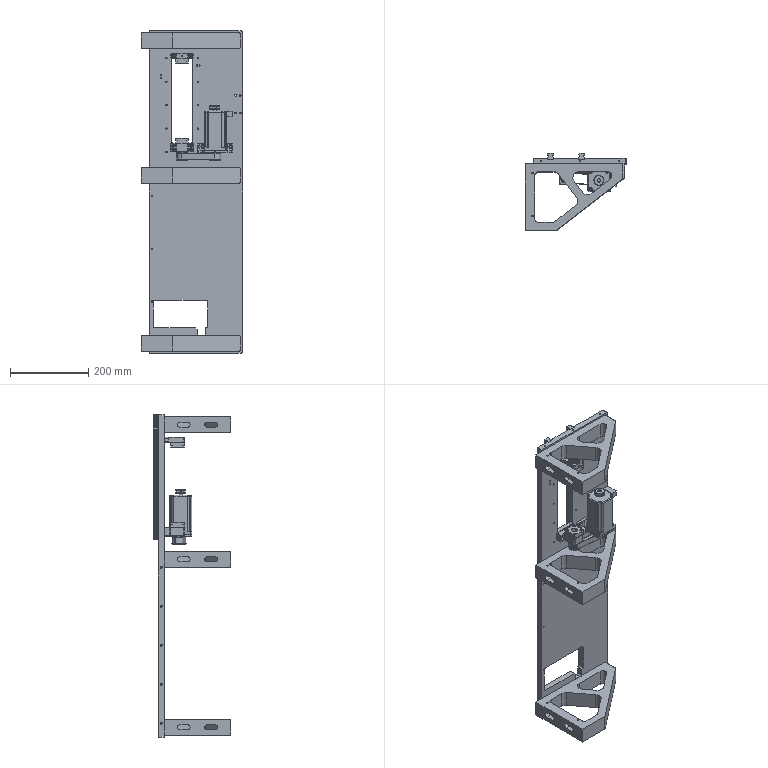Part | NX | features BREP 14 | 23 solids | 3138 faces | volume 5016669 mm3 | plane 1313 | cylinder 1283 | cone 242 | sphere 200 | torus 100 | commonest cylinder face diameters 25 x375 0.34 x138 3.3 x124 2.06 x80 24.07 x52 2.5 x42